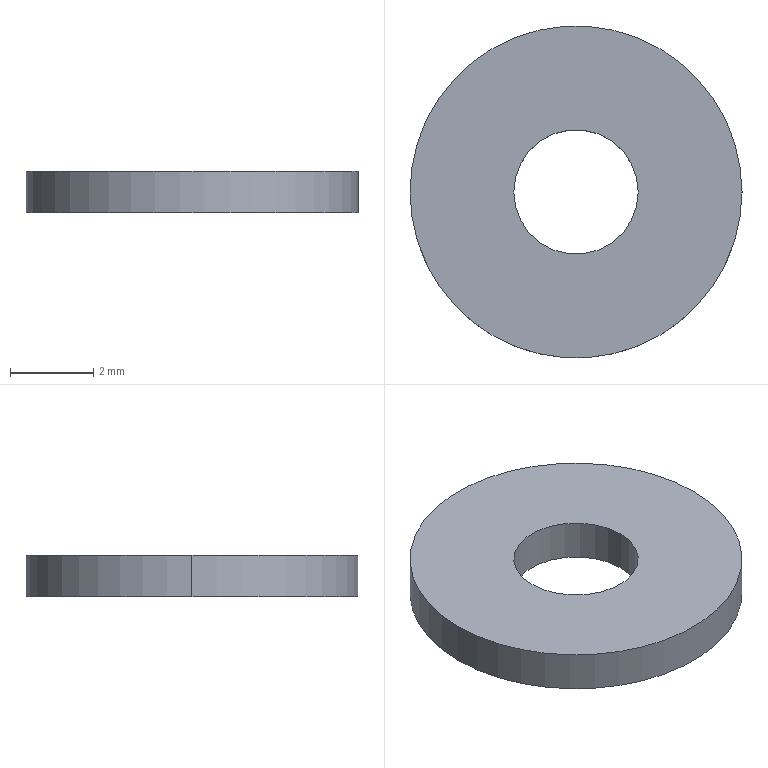Part | SolidWorks | features Attribute 1, Extrusion 1 | 1 solid | 6 faces | box 8 x 8 x 1 mm | volume 43.197 mm3 | cylinder 4 | plane 2 | commonest cylinder face diameters 3 x2 8 x2
STEP:
#1=CARTESIAN_POINT('',(-1.5,0.,1.));
#2=VERTEX_POINT('',#1);
#3=CARTESIAN_POINT('',(1.5,0.,1.));
#4=VERTEX_POINT('',#3);
#5=CARTESIAN_POINT('',(0.,0.,1.));
#6=DIRECTION('',(0.,0.,1.));
#7=DIRECTION('',(1.,0.,0.));
#8=AXIS2_PLACEMENT_3D('',#5,#6,#7);
#9=CIRCLE('',#8,1.5);
#10=EDGE_CURVE('',#2,#4,#9,.T.);
#11=ORIENTED_EDGE('',*,*,#10,.T.);
#12=CARTESIAN_POINT('',(1.5,0.,0.));
#13=VERTEX_POINT('',#12);
#14=CARTESIAN_POINT('',(1.5,0.,1.));
#15=DIRECTION('',(0.,0.,-1.));
#16=VECTOR('',#15,1000.);
#17=LINE('',#14,#16);
#18=EDGE_CURVE('',#4,#13,#17,.T.);
#19=ORIENTED_EDGE('',*,*,#18,.T.);
#20=CARTESIAN_POINT('',(-1.5,0.,0.));
#21=VERTEX_POINT('',#20);
#22=CARTESIAN_POINT('',(0.,0.,0.));
#23=DIRECTION('',(0.,0.,1.));
#24=DIRECTION('',(1.,0.,0.));
#25=AXIS2_PLACEMENT_3D('',#22,#23,#24);
#26=CIRCLE('',#25,1.5);
#27=EDGE_CURVE('',#21,#13,#26,.T.);
#28=ORIENTED_EDGE('',*,*,#27,.F.);
#29=CARTESIAN_POINT('',(-1.5,0.,1.));
#30=DIRECTION('',(0.,0.,-1.));
#31=VECTOR('',#30,1000.);
#32=LINE('',#29,#31);
#33=EDGE_CURVE('',#2,#21,#32,.T.);
#34=ORIENTED_EDGE('',*,*,#33,.F.);
#35=EDGE_LOOP('',(#11,#19,#28,#34));
#36=FACE_OUTER_BOUND('',#35,.T.);
#37=CARTESIAN_POINT('',(0.,0.,1.));
#38=DIRECTION('',(0.,0.,-1.));
#39=DIRECTION('',(-1.,0.,0.));
#40=AXIS2_PLACEMENT_3D('',#37,#38,#39);
#41=CYLINDRICAL_SURFACE('',#40,1.5);
#42=ADVANCED_FACE('',(#36),#41,.F.);
#43=CARTESIAN_POINT('',(4.,0.,1.));
#44=VERTEX_POINT('',#43);
#45=CARTESIAN_POINT('',(-4.,0.,1.));
#46=VERTEX_POINT('',#45);
#47=CARTESIAN_POINT('',(0.,0.,1.));
#48=DIRECTION('',(0.,0.,1.));
#49=DIRECTION('',(1.,0.,0.));
#50=AXIS2_PLACEMENT_3D('',#47,#48,#49);
#51=CIRCLE('',#50,4.);
#52=EDGE_CURVE('',#44,#46,#51,.T.);
#53=ORIENTED_EDGE('',*,*,#52,.F.);
#54=CARTESIAN_POINT('',(4.,0.,0.));
#55=VERTEX_POINT('',#54);
#56=CARTESIAN_POINT('',(4.,0.,1.));
#57=DIRECTION('',(0.,0.,-1.));
#58=VECTOR('',#57,1000.);
#59=LINE('',#56,#58);
#60=EDGE_CURVE('',#44,#55,#59,.T.);
#61=ORIENTED_EDGE('',*,*,#60,.T.);
#62=CARTESIAN_POINT('',(-4.,0.,0.));
#63=VERTEX_POINT('',#62);
#64=CARTESIAN_POINT('',(0.,0.,0.));
#65=DIRECTION('',(0.,0.,1.));
#66=DIRECTION('',(1.,0.,0.));
#67=AXIS2_PLACEMENT_3D('',#64,#65,#66);
#68=CIRCLE('',#67,4.);
#69=EDGE_CURVE('',#55,#63,#68,.T.);
#70=ORIENTED_EDGE('',*,*,#69,.T.);
#71=CARTESIAN_POINT('',(-4.,0.,1.));
#72=DIRECTION('',(0.,0.,-1.));
#73=VECTOR('',#72,1000.);
#74=LINE('',#71,#73);
#75=EDGE_CURVE('',#46,#63,#74,.T.);
#76=ORIENTED_EDGE('',*,*,#75,.F.);
#77=EDGE_LOOP('',(#53,#61,#70,#76));
#78=FACE_OUTER_BOUND('',#77,.T.);
#79=CARTESIAN_POINT('',(0.,0.,1.));
#80=DIRECTION('',(0.,0.,-1.));
#81=DIRECTION('',(-1.,0.,0.));
#82=AXIS2_PLACEMENT_3D('',#79,#80,#81);
#83=CYLINDRICAL_SURFACE('',#82,4.);
#84=ADVANCED_FACE('',(#78),#83,.T.);
#85=CARTESIAN_POINT('',(0.,0.,1.));
#86=DIRECTION('',(0.,0.,1.));
#87=DIRECTION('',(1.,0.,0.));
#88=AXIS2_PLACEMENT_3D('',#85,#86,#87);
#89=CIRCLE('',#88,4.);
#90=EDGE_CURVE('',#46,#44,#89,.T.);
#91=ORIENTED_EDGE('',*,*,#90,.T.);
#92=ORIENTED_EDGE('',*,*,#52,.T.);
#93=EDGE_LOOP('',(#91,#92));
#94=FACE_OUTER_BOUND('',#93,.T.);
#95=ORIENTED_EDGE('',*,*,#10,.F.);
#96=CARTESIAN_POINT('',(0.,0.,1.));
#97=DIRECTION('',(0.,0.,1.));
#98=DIRECTION('',(1.,0.,0.));
#99=AXIS2_PLACEMENT_3D('',#96,#97,#98);
#100=CIRCLE('',#99,1.5);
#101=EDGE_CURVE('',#4,#2,#100,.T.);
#102=ORIENTED_EDGE('',*,*,#101,.F.);
#103=EDGE_LOOP('',(#95,#102));
#104=FACE_BOUND('',#103,.T.);
#105=CARTESIAN_POINT('',(0.,0.,1.));
#106=DIRECTION('',(0.,0.,1.));
#107=DIRECTION('',(1.,0.,0.));
#108=AXIS2_PLACEMENT_3D('',#105,#106,#107);
#109=PLANE('',#108);
#110=ADVANCED_FACE('',(#94,#104),#109,.T.);
#111=CARTESIAN_POINT('',(0.,0.,0.));
#112=DIRECTION('',(0.,0.,1.));
#113=DIRECTION('',(1.,0.,0.));
#114=AXIS2_PLACEMENT_3D('',#111,#112,#113);
#115=CIRCLE('',#114,4.);
#116=EDGE_CURVE('',#63,#55,#115,.T.);
#117=ORIENTED_EDGE('',*,*,#116,.F.);
#118=ORIENTED_EDGE('',*,*,#69,.F.);
#119=EDGE_LOOP('',(#117,#118));
#120=FACE_OUTER_BOUND('',#119,.T.);
#121=ORIENTED_EDGE('',*,*,#27,.T.);
#122=CARTESIAN_POINT('',(0.,0.,0.));
#123=DIRECTION('',(0.,0.,1.));
#124=DIRECTION('',(1.,0.,0.));
#125=AXIS2_PLACEMENT_3D('',#122,#123,#124);
#126=CIRCLE('',#125,1.5);
#127=EDGE_CURVE('',#13,#21,#126,.T.);
#128=ORIENTED_EDGE('',*,*,#127,.T.);
#129=EDGE_LOOP('',(#121,#128));
#130=FACE_BOUND('',#129,.T.);
#131=CARTESIAN_POINT('',(0.,0.,0.));
#132=DIRECTION('',(0.,0.,1.));
#133=DIRECTION('',(1.,0.,0.));
#134=AXIS2_PLACEMENT_3D('',#131,#132,#133);
#135=PLANE('',#134);
#136=ADVANCED_FACE('',(#120,#130),#135,.F.);
#137=ORIENTED_EDGE('',*,*,#60,.F.);
#138=ORIENTED_EDGE('',*,*,#90,.F.);
#139=ORIENTED_EDGE('',*,*,#75,.T.);
#140=ORIENTED_EDGE('',*,*,#116,.T.);
#141=EDGE_LOOP('',(#137,#138,#139,#140));
#142=FACE_OUTER_BOUND('',#141,.T.);
#143=CARTESIAN_POINT('',(0.,0.,1.));
#144=DIRECTION('',(0.,0.,-1.));
#145=DIRECTION('',(-1.,0.,0.));
#146=AXIS2_PLACEMENT_3D('',#143,#144,#145);
#147=CYLINDRICAL_SURFACE('',#146,4.);
#148=ADVANCED_FACE('',(#142),#147,.T.);
#149=ORIENTED_EDGE('',*,*,#18,.F.);
#150=ORIENTED_EDGE('',*,*,#101,.T.);
#151=ORIENTED_EDGE('',*,*,#33,.T.);
#152=ORIENTED_EDGE('',*,*,#127,.F.);
#153=EDGE_LOOP('',(#149,#150,#151,#152));
#154=FACE_OUTER_BOUND('',#153,.T.);
#155=CARTESIAN_POINT('',(0.,0.,1.));
#156=DIRECTION('',(0.,0.,-1.));
#157=DIRECTION('',(-1.,0.,0.));
#158=AXIS2_PLACEMENT_3D('',#155,#156,#157);
#159=CYLINDRICAL_SURFACE('',#158,1.5);
#160=ADVANCED_FACE('',(#154),#159,.F.);
#161=CLOSED_SHELL('',(#42,#84,#110,#136,#148,#160));
#162=MANIFOLD_SOLID_BREP('',#161);
#163=CARTESIAN_POINT('',(0.,0.,0.));
#164=DIRECTION('',(0.,0.,1.));
#165=DIRECTION('',(1.,0.,0.));
#166=AXIS2_PLACEMENT_3D('',#163,#164,#165);
#167=(LENGTH_UNIT()NAMED_UNIT(*)SI_UNIT(.MILLI.,.METRE.));
#168=UNCERTAINTY_MEASURE_WITH_UNIT(LENGTH_MEASURE(0.00001),#167,'','');
#169=(NAMED_UNIT(*)PLANE_ANGLE_UNIT()SI_UNIT($,.RADIAN.));
#170=(NAMED_UNIT(*)SI_UNIT($,.STERADIAN.)SOLID_ANGLE_UNIT());
#171=(GEOMETRIC_REPRESENTATION_CONTEXT(3)GLOBAL_UNCERTAINTY_ASSIGNED_CONTEXT((#168))GLOBAL_UNIT_ASSIGNED_CONTEXT((#167,#169,#170))REPRESENTATION_CONTEXT('',''));
#172=ADVANCED_BREP_SHAPE_REPRESENTATION('',(#162,#166),#171);